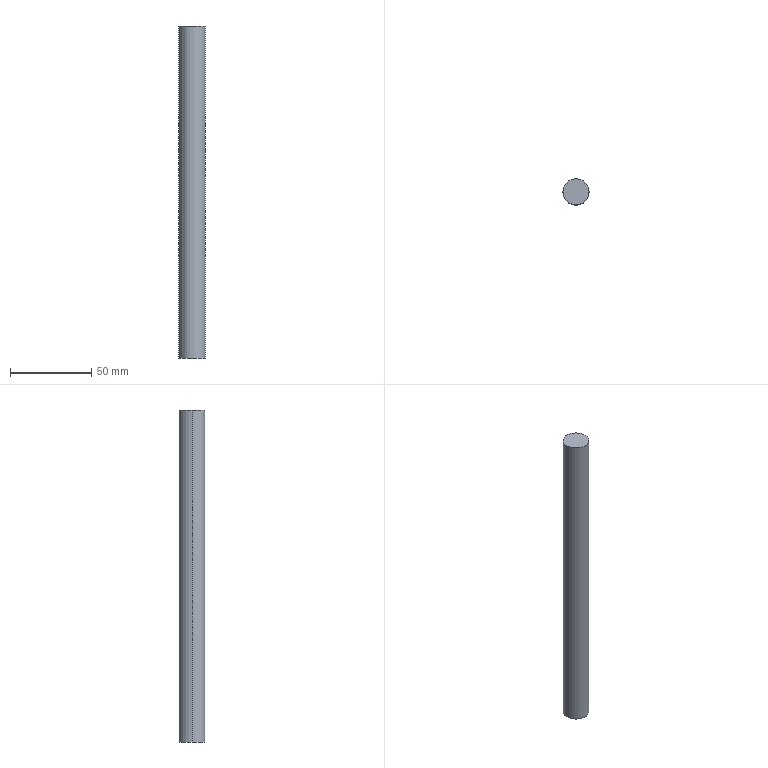Part | SolidWorks | features BaseBody 1 | 1 solid | 4 faces | box 16 x 16 x 204 mm | volume 41017 mm3 | cylinder 2 | plane 2 | commonest cylinder face diameters 16 x2
STEP:
#1=CARTESIAN_POINT('',(8.,0.,0.));
#2=VERTEX_POINT('',#1);
#3=CARTESIAN_POINT('',(-8.,0.,0.));
#4=VERTEX_POINT('',#3);
#5=CARTESIAN_POINT('',(0.,0.,0.));
#6=DIRECTION('',(0.,0.,1.));
#7=DIRECTION('',(1.,0.,0.));
#8=AXIS2_PLACEMENT_3D('',#5,#6,#7);
#9=CIRCLE('',#8,8.);
#10=EDGE_CURVE('',#2,#4,#9,.T.);
#11=ORIENTED_EDGE('',*,*,#10,.F.);
#12=CARTESIAN_POINT('',(8.,0.,-204.));
#13=VERTEX_POINT('',#12);
#14=CARTESIAN_POINT('',(8.,0.,0.));
#15=DIRECTION('',(0.,0.,-1.));
#16=VECTOR('',#15,1000.);
#17=LINE('',#14,#16);
#18=EDGE_CURVE('',#2,#13,#17,.T.);
#19=ORIENTED_EDGE('',*,*,#18,.T.);
#20=CARTESIAN_POINT('',(-8.,0.,-204.));
#21=VERTEX_POINT('',#20);
#22=CARTESIAN_POINT('',(0.,0.,-204.));
#23=DIRECTION('',(0.,0.,1.));
#24=DIRECTION('',(1.,0.,0.));
#25=AXIS2_PLACEMENT_3D('',#22,#23,#24);
#26=CIRCLE('',#25,8.);
#27=EDGE_CURVE('',#13,#21,#26,.T.);
#28=ORIENTED_EDGE('',*,*,#27,.T.);
#29=CARTESIAN_POINT('',(-8.,0.,0.));
#30=DIRECTION('',(0.,0.,-1.));
#31=VECTOR('',#30,1000.);
#32=LINE('',#29,#31);
#33=EDGE_CURVE('',#4,#21,#32,.T.);
#34=ORIENTED_EDGE('',*,*,#33,.F.);
#35=EDGE_LOOP('',(#11,#19,#28,#34));
#36=FACE_OUTER_BOUND('',#35,.T.);
#37=CARTESIAN_POINT('',(0.,0.,0.));
#38=DIRECTION('',(0.,0.,-1.));
#39=DIRECTION('',(-1.,0.,0.));
#40=AXIS2_PLACEMENT_3D('',#37,#38,#39);
#41=CYLINDRICAL_SURFACE('',#40,8.);
#42=ADVANCED_FACE('',(#36),#41,.T.);
#43=ORIENTED_EDGE('',*,*,#18,.F.);
#44=CARTESIAN_POINT('',(0.,0.,0.));
#45=DIRECTION('',(0.,0.,1.));
#46=DIRECTION('',(1.,0.,0.));
#47=AXIS2_PLACEMENT_3D('',#44,#45,#46);
#48=CIRCLE('',#47,8.);
#49=EDGE_CURVE('',#4,#2,#48,.T.);
#50=ORIENTED_EDGE('',*,*,#49,.F.);
#51=ORIENTED_EDGE('',*,*,#33,.T.);
#52=CARTESIAN_POINT('',(0.,0.,-204.));
#53=DIRECTION('',(0.,0.,1.));
#54=DIRECTION('',(1.,0.,0.));
#55=AXIS2_PLACEMENT_3D('',#52,#53,#54);
#56=CIRCLE('',#55,8.);
#57=EDGE_CURVE('',#21,#13,#56,.T.);
#58=ORIENTED_EDGE('',*,*,#57,.T.);
#59=EDGE_LOOP('',(#43,#50,#51,#58));
#60=FACE_OUTER_BOUND('',#59,.T.);
#61=CARTESIAN_POINT('',(0.,0.,0.));
#62=DIRECTION('',(0.,0.,-1.));
#63=DIRECTION('',(-1.,0.,0.));
#64=AXIS2_PLACEMENT_3D('',#61,#62,#63);
#65=CYLINDRICAL_SURFACE('',#64,8.);
#66=ADVANCED_FACE('',(#60),#65,.T.);
#67=ORIENTED_EDGE('',*,*,#49,.T.);
#68=ORIENTED_EDGE('',*,*,#10,.T.);
#69=EDGE_LOOP('',(#67,#68));
#70=FACE_OUTER_BOUND('',#69,.T.);
#71=CARTESIAN_POINT('',(0.,0.,0.));
#72=DIRECTION('',(0.,0.,1.));
#73=DIRECTION('',(1.,0.,0.));
#74=AXIS2_PLACEMENT_3D('',#71,#72,#73);
#75=PLANE('',#74);
#76=ADVANCED_FACE('',(#70),#75,.T.);
#77=ORIENTED_EDGE('',*,*,#57,.F.);
#78=ORIENTED_EDGE('',*,*,#27,.F.);
#79=EDGE_LOOP('',(#77,#78));
#80=FACE_OUTER_BOUND('',#79,.T.);
#81=CARTESIAN_POINT('',(0.,0.,-204.));
#82=DIRECTION('',(0.,0.,1.));
#83=DIRECTION('',(1.,0.,0.));
#84=AXIS2_PLACEMENT_3D('',#81,#82,#83);
#85=PLANE('',#84);
#86=ADVANCED_FACE('',(#80),#85,.F.);
#87=CLOSED_SHELL('',(#42,#66,#76,#86));
#88=MANIFOLD_SOLID_BREP('',#87);
#89=CARTESIAN_POINT('',(0.,0.,0.));
#90=DIRECTION('',(0.,0.,1.));
#91=DIRECTION('',(1.,0.,0.));
#92=AXIS2_PLACEMENT_3D('',#89,#90,#91);
#93=(LENGTH_UNIT()NAMED_UNIT(*)SI_UNIT(.MILLI.,.METRE.));
#94=UNCERTAINTY_MEASURE_WITH_UNIT(LENGTH_MEASURE(0.00001),#93,'','');
#95=(NAMED_UNIT(*)PLANE_ANGLE_UNIT()SI_UNIT($,.RADIAN.));
#96=(NAMED_UNIT(*)SI_UNIT($,.STERADIAN.)SOLID_ANGLE_UNIT());
#97=(GEOMETRIC_REPRESENTATION_CONTEXT(3)GLOBAL_UNCERTAINTY_ASSIGNED_CONTEXT((#94))GLOBAL_UNIT_ASSIGNED_CONTEXT((#93,#95,#96))REPRESENTATION_CONTEXT('',''));
#98=ADVANCED_BREP_SHAPE_REPRESENTATION('',(#88,#92),#97);